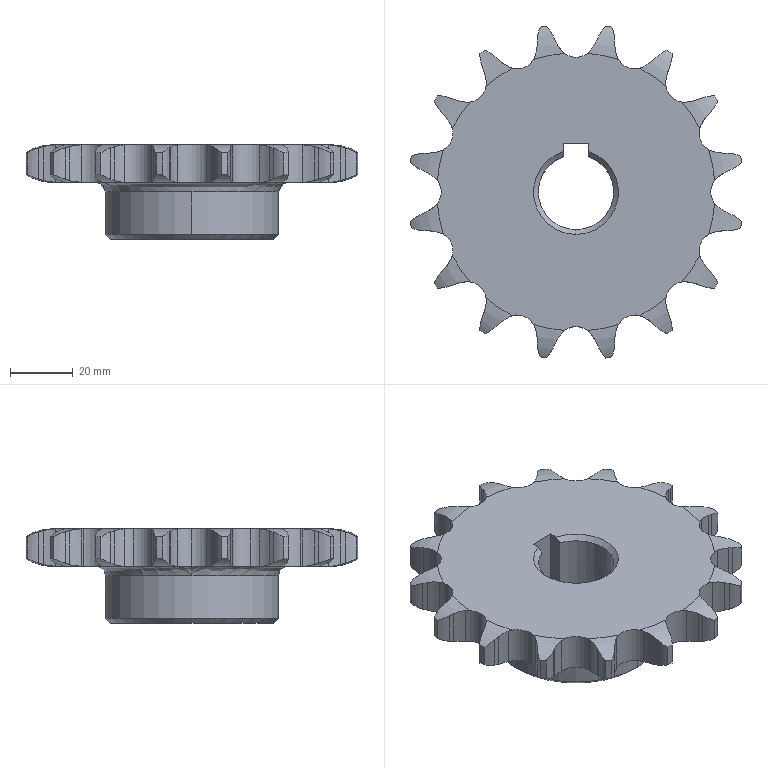Part | SolidWorks | features BaseBody 1 | 1 solid | 185 faces | box 105.504 x 105.504 x 30 mm | volume 109846 mm3 | cylinder 106 | plane 38 | spline 34 | cone 7 | commonest cylinder face diameters 19.857 x34 31.085 x32 12.029 x21 107.201 x16 55 x2 24 x1